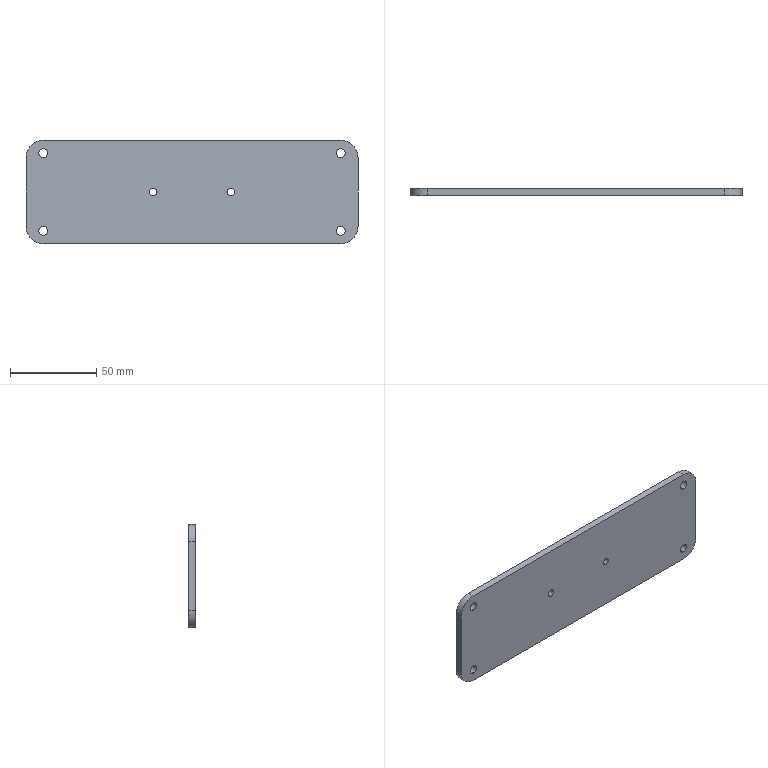Part | SolidWorks | features BaseBody 1 | 1 solid | 22 faces | box 193 x 4 x 60 mm | volume 45526 mm3 | cylinder 16 | plane 6 | commonest cylinder face diameters 5.2 x8 4.2 x4 20 x4
STEP:
#1=CARTESIAN_POINT('',(86.5,0.,-25.1));
#2=VERTEX_POINT('',#1);
#3=CARTESIAN_POINT('',(86.5,0.,-19.9));
#4=VERTEX_POINT('',#3);
#5=CARTESIAN_POINT('',(86.5,0.,-22.5));
#6=DIRECTION('',(0.,1.,0.));
#7=DIRECTION('',(0.,0.,1.));
#8=AXIS2_PLACEMENT_3D('',#5,#6,#7);
#9=CIRCLE('',#8,2.6);
#10=EDGE_CURVE('',#2,#4,#9,.T.);
#11=ORIENTED_EDGE('',*,*,#10,.F.);
#12=CARTESIAN_POINT('',(86.5,4.,-25.1));
#13=VERTEX_POINT('',#12);
#14=CARTESIAN_POINT('',(86.5,0.,-25.1));
#15=DIRECTION('',(0.,1.,0.));
#16=VECTOR('',#15,1000.);
#17=LINE('',#14,#16);
#18=EDGE_CURVE('',#2,#13,#17,.T.);
#19=ORIENTED_EDGE('',*,*,#18,.T.);
#20=CARTESIAN_POINT('',(86.5,4.,-19.9));
#21=VERTEX_POINT('',#20);
#22=CARTESIAN_POINT('',(86.5,4.,-22.5));
#23=DIRECTION('',(0.,1.,0.));
#24=DIRECTION('',(0.,0.,1.));
#25=AXIS2_PLACEMENT_3D('',#22,#23,#24);
#26=CIRCLE('',#25,2.6);
#27=EDGE_CURVE('',#13,#21,#26,.T.);
#28=ORIENTED_EDGE('',*,*,#27,.T.);
#29=CARTESIAN_POINT('',(86.5,0.,-19.9));
#30=DIRECTION('',(0.,1.,0.));
#31=VECTOR('',#30,1000.);
#32=LINE('',#29,#31);
#33=EDGE_CURVE('',#4,#21,#32,.T.);
#34=ORIENTED_EDGE('',*,*,#33,.F.);
#35=EDGE_LOOP('',(#11,#19,#28,#34));
#36=FACE_OUTER_BOUND('',#35,.T.);
#37=CARTESIAN_POINT('',(86.5,0.,-22.5));
#38=DIRECTION('',(0.,1.,0.));
#39=DIRECTION('',(0.,0.,1.));
#40=AXIS2_PLACEMENT_3D('',#37,#38,#39);
#41=CYLINDRICAL_SURFACE('',#40,2.6);
#42=ADVANCED_FACE('',(#36),#41,.F.);
#43=CARTESIAN_POINT('',(86.5,0.,19.9));
#44=VERTEX_POINT('',#43);
#45=CARTESIAN_POINT('',(86.5,0.,25.1));
#46=VERTEX_POINT('',#45);
#47=CARTESIAN_POINT('',(86.5,0.,22.5));
#48=DIRECTION('',(0.,1.,0.));
#49=DIRECTION('',(0.,0.,1.));
#50=AXIS2_PLACEMENT_3D('',#47,#48,#49);
#51=CIRCLE('',#50,2.6);
#52=EDGE_CURVE('',#44,#46,#51,.T.);
#53=ORIENTED_EDGE('',*,*,#52,.F.);
#54=CARTESIAN_POINT('',(86.5,4.,19.9));
#55=VERTEX_POINT('',#54);
#56=CARTESIAN_POINT('',(86.5,0.,19.9));
#57=DIRECTION('',(0.,1.,0.));
#58=VECTOR('',#57,1000.);
#59=LINE('',#56,#58);
#60=EDGE_CURVE('',#44,#55,#59,.T.);
#61=ORIENTED_EDGE('',*,*,#60,.T.);
#62=CARTESIAN_POINT('',(86.5,4.,25.1));
#63=VERTEX_POINT('',#62);
#64=CARTESIAN_POINT('',(86.5,4.,22.5));
#65=DIRECTION('',(0.,1.,0.));
#66=DIRECTION('',(0.,0.,1.));
#67=AXIS2_PLACEMENT_3D('',#64,#65,#66);
#68=CIRCLE('',#67,2.6);
#69=EDGE_CURVE('',#55,#63,#68,.T.);
#70=ORIENTED_EDGE('',*,*,#69,.T.);
#71=CARTESIAN_POINT('',(86.5,0.,25.1));
#72=DIRECTION('',(0.,1.,0.));
#73=VECTOR('',#72,1000.);
#74=LINE('',#71,#73);
#75=EDGE_CURVE('',#46,#63,#74,.T.);
#76=ORIENTED_EDGE('',*,*,#75,.F.);
#77=EDGE_LOOP('',(#53,#61,#70,#76));
#78=FACE_OUTER_BOUND('',#77,.T.);
#79=CARTESIAN_POINT('',(86.5,0.,22.5));
#80=DIRECTION('',(0.,1.,0.));
#81=DIRECTION('',(0.,0.,1.));
#82=AXIS2_PLACEMENT_3D('',#79,#80,#81);
#83=CYLINDRICAL_SURFACE('',#82,2.6);
#84=ADVANCED_FACE('',(#78),#83,.F.);
#85=CARTESIAN_POINT('',(-86.5,0.,19.9));
#86=VERTEX_POINT('',#85);
#87=CARTESIAN_POINT('',(-86.5,0.,25.1));
#88=VERTEX_POINT('',#87);
#89=CARTESIAN_POINT('',(-86.5,0.,22.5));
#90=DIRECTION('',(0.,1.,0.));
#91=DIRECTION('',(0.,0.,1.));
#92=AXIS2_PLACEMENT_3D('',#89,#90,#91);
#93=CIRCLE('',#92,2.6);
#94=EDGE_CURVE('',#86,#88,#93,.T.);
#95=ORIENTED_EDGE('',*,*,#94,.F.);
#96=CARTESIAN_POINT('',(-86.5,4.,19.9));
#97=VERTEX_POINT('',#96);
#98=CARTESIAN_POINT('',(-86.5,0.,19.9));
#99=DIRECTION('',(0.,1.,0.));
#100=VECTOR('',#99,1000.);
#101=LINE('',#98,#100);
#102=EDGE_CURVE('',#86,#97,#101,.T.);
#103=ORIENTED_EDGE('',*,*,#102,.T.);
#104=CARTESIAN_POINT('',(-86.5,4.,25.1));
#105=VERTEX_POINT('',#104);
#106=CARTESIAN_POINT('',(-86.5,4.,22.5));
#107=DIRECTION('',(0.,1.,0.));
#108=DIRECTION('',(0.,0.,1.));
#109=AXIS2_PLACEMENT_3D('',#106,#107,#108);
#110=CIRCLE('',#109,2.6);
#111=EDGE_CURVE('',#97,#105,#110,.T.);
#112=ORIENTED_EDGE('',*,*,#111,.T.);
#113=CARTESIAN_POINT('',(-86.5,0.,25.1));
#114=DIRECTION('',(0.,1.,0.));
#115=VECTOR('',#114,1000.);
#116=LINE('',#113,#115);
#117=EDGE_CURVE('',#88,#105,#116,.T.);
#118=ORIENTED_EDGE('',*,*,#117,.F.);
#119=EDGE_LOOP('',(#95,#103,#112,#118));
#120=FACE_OUTER_BOUND('',#119,.T.);
#121=CARTESIAN_POINT('',(-86.5,0.,22.5));
#122=DIRECTION('',(0.,1.,0.));
#123=DIRECTION('',(0.,0.,1.));
#124=AXIS2_PLACEMENT_3D('',#121,#122,#123);
#125=CYLINDRICAL_SURFACE('',#124,2.6);
#126=ADVANCED_FACE('',(#120),#125,.F.);
#127=CARTESIAN_POINT('',(-86.5,0.,-25.1));
#128=VERTEX_POINT('',#127);
#129=CARTESIAN_POINT('',(-86.5,0.,-19.9));
#130=VERTEX_POINT('',#129);
#131=CARTESIAN_POINT('',(-86.5,0.,-22.5));
#132=DIRECTION('',(0.,1.,0.));
#133=DIRECTION('',(0.,0.,1.));
#134=AXIS2_PLACEMENT_3D('',#131,#132,#133);
#135=CIRCLE('',#134,2.6);
#136=EDGE_CURVE('',#128,#130,#135,.T.);
#137=ORIENTED_EDGE('',*,*,#136,.F.);
#138=CARTESIAN_POINT('',(-86.5,4.,-25.1));
#139=VERTEX_POINT('',#138);
#140=CARTESIAN_POINT('',(-86.5,0.,-25.1));
#141=DIRECTION('',(0.,1.,0.));
#142=VECTOR('',#141,1000.);
#143=LINE('',#140,#142);
#144=EDGE_CURVE('',#128,#139,#143,.T.);
#145=ORIENTED_EDGE('',*,*,#144,.T.);
#146=CARTESIAN_POINT('',(-86.5,4.,-19.9));
#147=VERTEX_POINT('',#146);
#148=CARTESIAN_POINT('',(-86.5,4.,-22.5));
#149=DIRECTION('',(0.,1.,0.));
#150=DIRECTION('',(0.,0.,1.));
#151=AXIS2_PLACEMENT_3D('',#148,#149,#150);
#152=CIRCLE('',#151,2.6);
#153=EDGE_CURVE('',#139,#147,#152,.T.);
#154=ORIENTED_EDGE('',*,*,#153,.T.);
#155=CARTESIAN_POINT('',(-86.5,0.,-19.9));
#156=DIRECTION('',(0.,1.,0.));
#157=VECTOR('',#156,1000.);
#158=LINE('',#155,#157);
#159=EDGE_CURVE('',#130,#147,#158,.T.);
#160=ORIENTED_EDGE('',*,*,#159,.F.);
#161=EDGE_LOOP('',(#137,#145,#154,#160));
#162=FACE_OUTER_BOUND('',#161,.T.);
#163=CARTESIAN_POINT('',(-86.5,0.,-22.5));
#164=DIRECTION('',(0.,1.,0.));
#165=DIRECTION('',(0.,0.,1.));
#166=AXIS2_PLACEMENT_3D('',#163,#164,#165);
#167=CYLINDRICAL_SURFACE('',#166,2.6);
#168=ADVANCED_FACE('',(#162),#167,.F.);
#169=CARTESIAN_POINT('',(-22.5,0.,-2.1));
#170=VERTEX_POINT('',#169);
#171=CARTESIAN_POINT('',(-22.5,0.,2.1));
#172=VERTEX_POINT('',#171);
#173=CARTESIAN_POINT('',(-22.5,0.,0.));
#174=DIRECTION('',(0.,1.,0.));
#175=DIRECTION('',(0.,0.,1.));
#176=AXIS2_PLACEMENT_3D('',#173,#174,#175);
#177=CIRCLE('',#176,2.1);
#178=EDGE_CURVE('',#170,#172,#177,.T.);
#179=ORIENTED_EDGE('',*,*,#178,.F.);
#180=CARTESIAN_POINT('',(-22.5,4.,-2.1));
#181=VERTEX_POINT('',#180);
#182=CARTESIAN_POINT('',(-22.5,0.,-2.1));
#183=DIRECTION('',(0.,1.,0.));
#184=VECTOR('',#183,1000.);
#185=LINE('',#182,#184);
#186=EDGE_CURVE('',#170,#181,#185,.T.);
#187=ORIENTED_EDGE('',*,*,#186,.T.);
#188=CARTESIAN_POINT('',(-22.5,4.,2.1));
#189=VERTEX_POINT('',#188);
#190=CARTESIAN_POINT('',(-22.5,4.,0.));
#191=DIRECTION('',(0.,1.,0.));
#192=DIRECTION('',(0.,0.,1.));
#193=AXIS2_PLACEMENT_3D('',#190,#191,#192);
#194=CIRCLE('',#193,2.1);
#195=EDGE_CURVE('',#181,#189,#194,.T.);
#196=ORIENTED_EDGE('',*,*,#195,.T.);
#197=CARTESIAN_POINT('',(-22.5,0.,2.1));
#198=DIRECTION('',(0.,1.,0.));
#199=VECTOR('',#198,1000.);
#200=LINE('',#197,#199);
#201=EDGE_CURVE('',#172,#189,#200,.T.);
#202=ORIENTED_EDGE('',*,*,#201,.F.);
#203=EDGE_LOOP('',(#179,#187,#196,#202));
#204=FACE_OUTER_BOUND('',#203,.T.);
#205=CARTESIAN_POINT('',(-22.5,0.,0.));
#206=DIRECTION('',(0.,1.,0.));
#207=DIRECTION('',(0.,0.,1.));
#208=AXIS2_PLACEMENT_3D('',#205,#206,#207);
#209=CYLINDRICAL_SURFACE('',#208,2.1);
#210=ADVANCED_FACE('',(#204),#209,.F.);
#211=CARTESIAN_POINT('',(22.5,0.,-2.1));
#212=VERTEX_POINT('',#211);
#213=CARTESIAN_POINT('',(22.5,0.,2.1));
#214=VERTEX_POINT('',#213);
#215=CARTESIAN_POINT('',(22.5,0.,0.));
#216=DIRECTION('',(0.,1.,0.));
#217=DIRECTION('',(0.,0.,1.));
#218=AXIS2_PLACEMENT_3D('',#215,#216,#217);
#219=CIRCLE('',#218,2.1);
#220=EDGE_CURVE('',#212,#214,#219,.T.);
#221=ORIENTED_EDGE('',*,*,#220,.F.);
#222=CARTESIAN_POINT('',(22.5,4.,-2.1));
#223=VERTEX_POINT('',#222);
#224=CARTESIAN_POINT('',(22.5,0.,-2.1));
#225=DIRECTION('',(0.,1.,0.));
#226=VECTOR('',#225,1000.);
#227=LINE('',#224,#226);
#228=EDGE_CURVE('',#212,#223,#227,.T.);
#229=ORIENTED_EDGE('',*,*,#228,.T.);
#230=CARTESIAN_POINT('',(22.5,4.,2.1));
#231=VERTEX_POINT('',#230);
#232=CARTESIAN_POINT('',(22.5,4.,0.));
#233=DIRECTION('',(0.,1.,0.));
#234=DIRECTION('',(0.,0.,1.));
#235=AXIS2_PLACEMENT_3D('',#232,#233,#234);
#236=CIRCLE('',#235,2.1);
#237=EDGE_CURVE('',#223,#231,#236,.T.);
#238=ORIENTED_EDGE('',*,*,#237,.T.);
#239=CARTESIAN_POINT('',(22.5,0.,2.1));
#240=DIRECTION('',(0.,1.,0.));
#241=VECTOR('',#240,1000.);
#242=LINE('',#239,#241);
#243=EDGE_CURVE('',#214,#231,#242,.T.);
#244=ORIENTED_EDGE('',*,*,#243,.F.);
#245=EDGE_LOOP('',(#221,#229,#238,#244));
#246=FACE_OUTER_BOUND('',#245,.T.);
#247=CARTESIAN_POINT('',(22.5,0.,0.));
#248=DIRECTION('',(0.,1.,0.));
#249=DIRECTION('',(0.,0.,1.));
#250=AXIS2_PLACEMENT_3D('',#247,#248,#249);
#251=CYLINDRICAL_SURFACE('',#250,2.1);
#252=ADVANCED_FACE('',(#246),#251,.F.);
#253=CARTESIAN_POINT('',(96.5,4.,20.));
#254=VERTEX_POINT('',#253);
#255=CARTESIAN_POINT('',(86.5,4.,30.));
#256=VERTEX_POINT('',#255);
#257=CARTESIAN_POINT('',(86.5,4.,20.));
#258=DIRECTION('',(0.,-1.,0.));
#259=DIRECTION('',(0.,0.,-1.));
#260=AXIS2_PLACEMENT_3D('',#257,#258,#259);
#261=CIRCLE('',#260,10.);
#262=EDGE_CURVE('',#254,#256,#261,.T.);
#263=ORIENTED_EDGE('',*,*,#262,.F.);
#264=CARTESIAN_POINT('',(96.5,4.,-20.));
#265=VERTEX_POINT('',#264);
#266=CARTESIAN_POINT('',(96.5,4.,0.));
#267=DIRECTION('',(0.,0.,1.));
#268=VECTOR('',#267,1000.);
#269=LINE('',#266,#268);
#270=EDGE_CURVE('',#265,#254,#269,.T.);
#271=ORIENTED_EDGE('',*,*,#270,.F.);
#272=CARTESIAN_POINT('',(86.5,4.,-30.));
#273=VERTEX_POINT('',#272);
#274=CARTESIAN_POINT('',(86.5,4.,-20.));
#275=DIRECTION('',(0.,-1.,0.));
#276=DIRECTION('',(0.,0.,-1.));
#277=AXIS2_PLACEMENT_3D('',#274,#275,#276);
#278=CIRCLE('',#277,10.);
#279=EDGE_CURVE('',#273,#265,#278,.T.);
#280=ORIENTED_EDGE('',*,*,#279,.F.);
#281=CARTESIAN_POINT('',(-86.5,4.,-30.));
#282=VERTEX_POINT('',#281);
#283=CARTESIAN_POINT('',(0.,4.,-30.));
#284=DIRECTION('',(1.,0.,0.));
#285=VECTOR('',#284,1000.);
#286=LINE('',#283,#285);
#287=EDGE_CURVE('',#282,#273,#286,.T.);
#288=ORIENTED_EDGE('',*,*,#287,.F.);
#289=CARTESIAN_POINT('',(-96.5,4.,-20.));
#290=VERTEX_POINT('',#289);
#291=CARTESIAN_POINT('',(-86.5,4.,-20.));
#292=DIRECTION('',(0.,-1.,0.));
#293=DIRECTION('',(0.,0.,-1.));
#294=AXIS2_PLACEMENT_3D('',#291,#292,#293);
#295=CIRCLE('',#294,10.);
#296=EDGE_CURVE('',#290,#282,#295,.T.);
#297=ORIENTED_EDGE('',*,*,#296,.F.);
#298=CARTESIAN_POINT('',(-96.5,4.,20.));
#299=VERTEX_POINT('',#298);
#300=CARTESIAN_POINT('',(-96.5,4.,0.));
#301=DIRECTION('',(0.,0.,-1.));
#302=VECTOR('',#301,1000.);
#303=LINE('',#300,#302);
#304=EDGE_CURVE('',#299,#290,#303,.T.);
#305=ORIENTED_EDGE('',*,*,#304,.F.);
#306=CARTESIAN_POINT('',(-86.5,4.,30.));
#307=VERTEX_POINT('',#306);
#308=CARTESIAN_POINT('',(-86.5,4.,20.));
#309=DIRECTION('',(0.,-1.,0.));
#310=DIRECTION('',(0.,0.,-1.));
#311=AXIS2_PLACEMENT_3D('',#308,#309,#310);
#312=CIRCLE('',#311,10.);
#313=EDGE_CURVE('',#307,#299,#312,.T.);
#314=ORIENTED_EDGE('',*,*,#313,.F.);
#315=CARTESIAN_POINT('',(0.,4.,30.));
#316=DIRECTION('',(-1.,0.,0.));
#317=VECTOR('',#316,1000.);
#318=LINE('',#315,#317);
#319=EDGE_CURVE('',#256,#307,#318,.T.);
#320=ORIENTED_EDGE('',*,*,#319,.F.);
#321=EDGE_LOOP('',(#263,#271,#280,#288,#297,#305,#314,#320));
#322=FACE_OUTER_BOUND('',#321,.T.);
#323=CARTESIAN_POINT('',(86.5,4.,-22.5));
#324=DIRECTION('',(0.,1.,0.));
#325=DIRECTION('',(0.,0.,1.));
#326=AXIS2_PLACEMENT_3D('',#323,#324,#325);
#327=CIRCLE('',#326,2.6);
#328=EDGE_CURVE('',#21,#13,#327,.T.);
#329=ORIENTED_EDGE('',*,*,#328,.F.);
#330=ORIENTED_EDGE('',*,*,#27,.F.);
#331=EDGE_LOOP('',(#329,#330));
#332=FACE_BOUND('',#331,.T.);
#333=CARTESIAN_POINT('',(86.5,4.,22.5));
#334=DIRECTION('',(0.,1.,0.));
#335=DIRECTION('',(0.,0.,1.));
#336=AXIS2_PLACEMENT_3D('',#333,#334,#335);
#337=CIRCLE('',#336,2.6);
#338=EDGE_CURVE('',#63,#55,#337,.T.);
#339=ORIENTED_EDGE('',*,*,#338,.F.);
#340=ORIENTED_EDGE('',*,*,#69,.F.);
#341=EDGE_LOOP('',(#339,#340));
#342=FACE_BOUND('',#341,.T.);
#343=CARTESIAN_POINT('',(-86.5,4.,22.5));
#344=DIRECTION('',(0.,1.,0.));
#345=DIRECTION('',(0.,0.,1.));
#346=AXIS2_PLACEMENT_3D('',#343,#344,#345);
#347=CIRCLE('',#346,2.6);
#348=EDGE_CURVE('',#105,#97,#347,.T.);
#349=ORIENTED_EDGE('',*,*,#348,.F.);
#350=ORIENTED_EDGE('',*,*,#111,.F.);
#351=EDGE_LOOP('',(#349,#350));
#352=FACE_BOUND('',#351,.T.);
#353=CARTESIAN_POINT('',(-86.5,4.,-22.5));
#354=DIRECTION('',(0.,1.,0.));
#355=DIRECTION('',(0.,0.,1.));
#356=AXIS2_PLACEMENT_3D('',#353,#354,#355);
#357=CIRCLE('',#356,2.6);
#358=EDGE_CURVE('',#147,#139,#357,.T.);
#359=ORIENTED_EDGE('',*,*,#358,.F.);
#360=ORIENTED_EDGE('',*,*,#153,.F.);
#361=EDGE_LOOP('',(#359,#360));
#362=FACE_BOUND('',#361,.T.);
#363=CARTESIAN_POINT('',(-22.5,4.,0.));
#364=DIRECTION('',(0.,1.,0.));
#365=DIRECTION('',(0.,0.,1.));
#366=AXIS2_PLACEMENT_3D('',#363,#364,#365);
#367=CIRCLE('',#366,2.1);
#368=EDGE_CURVE('',#189,#181,#367,.T.);
#369=ORIENTED_EDGE('',*,*,#368,.F.);
#370=ORIENTED_EDGE('',*,*,#195,.F.);
#371=EDGE_LOOP('',(#369,#370));
#372=FACE_BOUND('',#371,.T.);
#373=CARTESIAN_POINT('',(22.5,4.,0.));
#374=DIRECTION('',(0.,1.,0.));
#375=DIRECTION('',(0.,0.,1.));
#376=AXIS2_PLACEMENT_3D('',#373,#374,#375);
#377=CIRCLE('',#376,2.1);
#378=EDGE_CURVE('',#231,#223,#377,.T.);
#379=ORIENTED_EDGE('',*,*,#378,.F.);
#380=ORIENTED_EDGE('',*,*,#237,.F.);
#381=EDGE_LOOP('',(#379,#380));
#382=FACE_BOUND('',#381,.T.);
#383=CARTESIAN_POINT('',(0.,4.,0.));
#384=DIRECTION('',(0.,-1.,0.));
#385=DIRECTION('',(0.,0.,-1.));
#386=AXIS2_PLACEMENT_3D('',#383,#384,#385);
#387=PLANE('',#386);
#388=ADVANCED_FACE('',(#322,#332,#342,#352,#362,#372,#382),#387,.F.);
#389=CARTESIAN_POINT('',(86.5,0.,30.));
#390=VERTEX_POINT('',#389);
#391=CARTESIAN_POINT('',(86.5,4.,30.));
#392=DIRECTION('',(0.,-1.,0.));
#393=VECTOR('',#392,1000.);
#394=LINE('',#391,#393);
#395=EDGE_CURVE('',#256,#390,#394,.T.);
#396=ORIENTED_EDGE('',*,*,#395,.F.);
#397=ORIENTED_EDGE('',*,*,#319,.T.);
#398=CARTESIAN_POINT('',(-86.5,0.,30.));
#399=VERTEX_POINT('',#398);
#400=CARTESIAN_POINT('',(-86.5,4.,30.));
#401=DIRECTION('',(0.,1.,0.));
#402=VECTOR('',#401,1000.);
#403=LINE('',#400,#402);
#404=EDGE_CURVE('',#399,#307,#403,.T.);
#405=ORIENTED_EDGE('',*,*,#404,.F.);
#406=CARTESIAN_POINT('',(-96.5,0.,30.));
#407=DIRECTION('',(-1.,0.,0.));
#408=VECTOR('',#407,1000.);
#409=LINE('',#406,#408);
#410=EDGE_CURVE('',#390,#399,#409,.T.);
#411=ORIENTED_EDGE('',*,*,#410,.F.);
#412=EDGE_LOOP('',(#396,#397,#405,#411));
#413=FACE_OUTER_BOUND('',#412,.T.);
#414=CARTESIAN_POINT('',(-96.5,4.,30.));
#415=DIRECTION('',(0.,0.,-1.));
#416=DIRECTION('',(-1.,0.,0.));
#417=AXIS2_PLACEMENT_3D('',#414,#415,#416);
#418=PLANE('',#417);
#419=ADVANCED_FACE('',(#413),#418,.F.);
#420=CARTESIAN_POINT('',(96.5,0.,20.));
#421=VERTEX_POINT('',#420);
#422=CARTESIAN_POINT('',(86.5,0.,20.));
#423=DIRECTION('',(0.,1.,0.));
#424=DIRECTION('',(0.,0.,-1.));
#425=AXIS2_PLACEMENT_3D('',#422,#423,#424);
#426=CIRCLE('',#425,10.);
#427=EDGE_CURVE('',#390,#421,#426,.T.);
#428=ORIENTED_EDGE('',*,*,#427,.T.);
#429=CARTESIAN_POINT('',(96.5,4.,20.));
#430=DIRECTION('',(0.,1.,0.));
#431=VECTOR('',#430,1000.);
#432=LINE('',#429,#431);
#433=EDGE_CURVE('',#421,#254,#432,.T.);
#434=ORIENTED_EDGE('',*,*,#433,.T.);
#435=ORIENTED_EDGE('',*,*,#262,.T.);
#436=ORIENTED_EDGE('',*,*,#395,.T.);
#437=EDGE_LOOP('',(#428,#434,#435,#436));
#438=FACE_OUTER_BOUND('',#437,.T.);
#439=CARTESIAN_POINT('',(86.5,4.,20.));
#440=DIRECTION('',(0.,-1.,0.));
#441=DIRECTION('',(0.,0.,-1.));
#442=AXIS2_PLACEMENT_3D('',#439,#440,#441);
#443=CYLINDRICAL_SURFACE('',#442,10.);
#444=ADVANCED_FACE('',(#438),#443,.T.);
#445=ORIENTED_EDGE('',*,*,#433,.F.);
#446=CARTESIAN_POINT('',(96.5,0.,-20.));
#447=VERTEX_POINT('',#446);
#448=CARTESIAN_POINT('',(96.5,0.,30.));
#449=DIRECTION('',(0.,0.,1.));
#450=VECTOR('',#449,1000.);
#451=LINE('',#448,#450);
#452=EDGE_CURVE('',#447,#421,#451,.T.);
#453=ORIENTED_EDGE('',*,*,#452,.F.);
#454=CARTESIAN_POINT('',(96.5,4.,-20.));
#455=DIRECTION('',(0.,-1.,0.));
#456=VECTOR('',#455,1000.);
#457=LINE('',#454,#456);
#458=EDGE_CURVE('',#265,#447,#457,.T.);
#459=ORIENTED_EDGE('',*,*,#458,.F.);
#460=ORIENTED_EDGE('',*,*,#270,.T.);
#461=EDGE_LOOP('',(#445,#453,#459,#460));
#462=FACE_OUTER_BOUND('',#461,.T.);
#463=CARTESIAN_POINT('',(96.5,4.,30.));
#464=DIRECTION('',(-1.,0.,0.));
#465=DIRECTION('',(0.,0.,1.));
#466=AXIS2_PLACEMENT_3D('',#463,#464,#465);
#467=PLANE('',#466);
#468=ADVANCED_FACE('',(#462),#467,.F.);
#469=CARTESIAN_POINT('',(86.5,0.,-30.));
#470=VERTEX_POINT('',#469);
#471=CARTESIAN_POINT('',(86.5,0.,-20.));
#472=DIRECTION('',(0.,1.,0.));
#473=DIRECTION('',(0.,0.,-1.));
#474=AXIS2_PLACEMENT_3D('',#471,#472,#473);
#475=CIRCLE('',#474,10.);
#476=EDGE_CURVE('',#447,#470,#475,.T.);
#477=ORIENTED_EDGE('',*,*,#476,.T.);
#478=CARTESIAN_POINT('',(86.5,4.,-30.));
#479=DIRECTION('',(0.,1.,0.));
#480=VECTOR('',#479,1000.);
#481=LINE('',#478,#480);
#482=EDGE_CURVE('',#470,#273,#481,.T.);
#483=ORIENTED_EDGE('',*,*,#482,.T.);
#484=ORIENTED_EDGE('',*,*,#279,.T.);
#485=ORIENTED_EDGE('',*,*,#458,.T.);
#486=EDGE_LOOP('',(#477,#483,#484,#485));
#487=FACE_OUTER_BOUND('',#486,.T.);
#488=CARTESIAN_POINT('',(86.5,4.,-20.));
#489=DIRECTION('',(0.,-1.,0.));
#490=DIRECTION('',(0.,0.,-1.));
#491=AXIS2_PLACEMENT_3D('',#488,#489,#490);
#492=CYLINDRICAL_SURFACE('',#491,10.);
#493=ADVANCED_FACE('',(#487),#492,.T.);
#494=ORIENTED_EDGE('',*,*,#482,.F.);
#495=CARTESIAN_POINT('',(-86.5,0.,-30.));
#496=VERTEX_POINT('',#495);
#497=CARTESIAN_POINT('',(-96.5,0.,-30.));
#498=DIRECTION('',(1.,0.,0.));
#499=VECTOR('',#498,1000.);
#500=LINE('',#497,#499);
#501=EDGE_CURVE('',#496,#470,#500,.T.);
#502=ORIENTED_EDGE('',*,*,#501,.F.);
#503=CARTESIAN_POINT('',(-86.5,4.,-30.));
#504=DIRECTION('',(0.,-1.,0.));
#505=VECTOR('',#504,1000.);
#506=LINE('',#503,#505);
#507=EDGE_CURVE('',#282,#496,#506,.T.);
#508=ORIENTED_EDGE('',*,*,#507,.F.);
#509=ORIENTED_EDGE('',*,*,#287,.T.);
#510=EDGE_LOOP('',(#494,#502,#508,#509));
#511=FACE_OUTER_BOUND('',#510,.T.);
#512=CARTESIAN_POINT('',(-96.5,4.,-30.));
#513=DIRECTION('',(0.,0.,1.));
#514=DIRECTION('',(1.,0.,0.));
#515=AXIS2_PLACEMENT_3D('',#512,#513,#514);
#516=PLANE('',#515);
#517=ADVANCED_FACE('',(#511),#516,.F.);
#518=CARTESIAN_POINT('',(-96.5,0.,-20.));
#519=VERTEX_POINT('',#518);
#520=CARTESIAN_POINT('',(-86.5,0.,-20.));
#521=DIRECTION('',(0.,1.,0.));
#522=DIRECTION('',(0.,0.,-1.));
#523=AXIS2_PLACEMENT_3D('',#520,#521,#522);
#524=CIRCLE('',#523,10.);
#525=EDGE_CURVE('',#496,#519,#524,.T.);
#526=ORIENTED_EDGE('',*,*,#525,.T.);
#527=CARTESIAN_POINT('',(-96.5,4.,-20.));
#528=DIRECTION('',(0.,1.,0.));
#529=VECTOR('',#528,1000.);
#530=LINE('',#527,#529);
#531=EDGE_CURVE('',#519,#290,#530,.T.);
#532=ORIENTED_EDGE('',*,*,#531,.T.);
#533=ORIENTED_EDGE('',*,*,#296,.T.);
#534=ORIENTED_EDGE('',*,*,#507,.T.);
#535=EDGE_LOOP('',(#526,#532,#533,#534));
#536=FACE_OUTER_BOUND('',#535,.T.);
#537=CARTESIAN_POINT('',(-86.5,4.,-20.));
#538=DIRECTION('',(0.,-1.,0.));
#539=DIRECTION('',(0.,0.,-1.));
#540=AXIS2_PLACEMENT_3D('',#537,#538,#539);
#541=CYLINDRICAL_SURFACE('',#540,10.);
#542=ADVANCED_FACE('',(#536),#541,.T.);
#543=CARTESIAN_POINT('',(-96.5,0.,20.));
#544=VERTEX_POINT('',#543);
#545=CARTESIAN_POINT('',(-96.5,4.,20.));
#546=DIRECTION('',(0.,-1.,0.));
#547=VECTOR('',#546,1000.);
#548=LINE('',#545,#547);
#549=EDGE_CURVE('',#299,#544,#548,.T.);
#550=ORIENTED_EDGE('',*,*,#549,.F.);
#551=ORIENTED_EDGE('',*,*,#304,.T.);
#552=ORIENTED_EDGE('',*,*,#531,.F.);
#553=CARTESIAN_POINT('',(-96.5,0.,30.));
#554=DIRECTION('',(0.,0.,-1.));
#555=VECTOR('',#554,1000.);
#556=LINE('',#553,#555);
#557=EDGE_CURVE('',#544,#519,#556,.T.);
#558=ORIENTED_EDGE('',*,*,#557,.F.);
#559=EDGE_LOOP('',(#550,#551,#552,#558));
#560=FACE_OUTER_BOUND('',#559,.T.);
#561=CARTESIAN_POINT('',(-96.5,4.,30.));
#562=DIRECTION('',(1.,0.,0.));
#563=DIRECTION('',(0.,0.,-1.));
#564=AXIS2_PLACEMENT_3D('',#561,#562,#563);
#565=PLANE('',#564);
#566=ADVANCED_FACE('',(#560),#565,.F.);
#567=CARTESIAN_POINT('',(-86.5,0.,20.));
#568=DIRECTION('',(0.,1.,0.));
#569=DIRECTION('',(0.,0.,-1.));
#570=AXIS2_PLACEMENT_3D('',#567,#568,#569);
#571=CIRCLE('',#570,10.);
#572=EDGE_CURVE('',#544,#399,#571,.T.);
#573=ORIENTED_EDGE('',*,*,#572,.T.);
#574=ORIENTED_EDGE('',*,*,#404,.T.);
#575=ORIENTED_EDGE('',*,*,#313,.T.);
#576=ORIENTED_EDGE('',*,*,#549,.T.);
#577=EDGE_LOOP('',(#573,#574,#575,#576));
#578=FACE_OUTER_BOUND('',#577,.T.);
#579=CARTESIAN_POINT('',(-86.5,4.,20.));
#580=DIRECTION('',(0.,-1.,0.));
#581=DIRECTION('',(0.,0.,-1.));
#582=AXIS2_PLACEMENT_3D('',#579,#580,#581);
#583=CYLINDRICAL_SURFACE('',#582,10.);
#584=ADVANCED_FACE('',(#578),#583,.T.);
#585=ORIENTED_EDGE('',*,*,#18,.F.);
#586=CARTESIAN_POINT('',(86.5,0.,-22.5));
#587=DIRECTION('',(0.,1.,0.));
#588=DIRECTION('',(0.,0.,1.));
#589=AXIS2_PLACEMENT_3D('',#586,#587,#588);
#590=CIRCLE('',#589,2.6);
#591=EDGE_CURVE('',#4,#2,#590,.T.);
#592=ORIENTED_EDGE('',*,*,#591,.F.);
#593=ORIENTED_EDGE('',*,*,#33,.T.);
#594=ORIENTED_EDGE('',*,*,#328,.T.);
#595=EDGE_LOOP('',(#585,#592,#593,#594));
#596=FACE_OUTER_BOUND('',#595,.T.);
#597=CARTESIAN_POINT('',(86.5,0.,-22.5));
#598=DIRECTION('',(0.,1.,0.));
#599=DIRECTION('',(0.,0.,1.));
#600=AXIS2_PLACEMENT_3D('',#597,#598,#599);
#601=CYLINDRICAL_SURFACE('',#600,2.6);
#602=ADVANCED_FACE('',(#596),#601,.F.);
#603=ORIENTED_EDGE('',*,*,#60,.F.);
#604=CARTESIAN_POINT('',(86.5,0.,22.5));
#605=DIRECTION('',(0.,1.,0.));
#606=DIRECTION('',(0.,0.,1.));
#607=AXIS2_PLACEMENT_3D('',#604,#605,#606);
#608=CIRCLE('',#607,2.6);
#609=EDGE_CURVE('',#46,#44,#608,.T.);
#610=ORIENTED_EDGE('',*,*,#609,.F.);
#611=ORIENTED_EDGE('',*,*,#75,.T.);
#612=ORIENTED_EDGE('',*,*,#338,.T.);
#613=EDGE_LOOP('',(#603,#610,#611,#612));
#614=FACE_OUTER_BOUND('',#613,.T.);
#615=CARTESIAN_POINT('',(86.5,0.,22.5));
#616=DIRECTION('',(0.,1.,0.));
#617=DIRECTION('',(0.,0.,1.));
#618=AXIS2_PLACEMENT_3D('',#615,#616,#617);
#619=CYLINDRICAL_SURFACE('',#618,2.6);
#620=ADVANCED_FACE('',(#614),#619,.F.);
#621=ORIENTED_EDGE('',*,*,#102,.F.);
#622=CARTESIAN_POINT('',(-86.5,0.,22.5));
#623=DIRECTION('',(0.,1.,0.));
#624=DIRECTION('',(0.,0.,1.));
#625=AXIS2_PLACEMENT_3D('',#622,#623,#624);
#626=CIRCLE('',#625,2.6);
#627=EDGE_CURVE('',#88,#86,#626,.T.);
#628=ORIENTED_EDGE('',*,*,#627,.F.);
#629=ORIENTED_EDGE('',*,*,#117,.T.);
#630=ORIENTED_EDGE('',*,*,#348,.T.);
#631=EDGE_LOOP('',(#621,#628,#629,#630));
#632=FACE_OUTER_BOUND('',#631,.T.);
#633=CARTESIAN_POINT('',(-86.5,0.,22.5));
#634=DIRECTION('',(0.,1.,0.));
#635=DIRECTION('',(0.,0.,1.));
#636=AXIS2_PLACEMENT_3D('',#633,#634,#635);
#637=CYLINDRICAL_SURFACE('',#636,2.6);
#638=ADVANCED_FACE('',(#632),#637,.F.);
#639=ORIENTED_EDGE('',*,*,#144,.F.);
#640=CARTESIAN_POINT('',(-86.5,0.,-22.5));
#641=DIRECTION('',(0.,1.,0.));
#642=DIRECTION('',(0.,0.,1.));
#643=AXIS2_PLACEMENT_3D('',#640,#641,#642);
#644=CIRCLE('',#643,2.6);
#645=EDGE_CURVE('',#130,#128,#644,.T.);
#646=ORIENTED_EDGE('',*,*,#645,.F.);
#647=ORIENTED_EDGE('',*,*,#159,.T.);
#648=ORIENTED_EDGE('',*,*,#358,.T.);
#649=EDGE_LOOP('',(#639,#646,#647,#648));
#650=FACE_OUTER_BOUND('',#649,.T.);
#651=CARTESIAN_POINT('',(-86.5,0.,-22.5));
#652=DIRECTION('',(0.,1.,0.));
#653=DIRECTION('',(0.,0.,1.));
#654=AXIS2_PLACEMENT_3D('',#651,#652,#653);
#655=CYLINDRICAL_SURFACE('',#654,2.6);
#656=ADVANCED_FACE('',(#650),#655,.F.);
#657=ORIENTED_EDGE('',*,*,#186,.F.);
#658=CARTESIAN_POINT('',(-22.5,0.,0.));
#659=DIRECTION('',(0.,1.,0.));
#660=DIRECTION('',(0.,0.,1.));
#661=AXIS2_PLACEMENT_3D('',#658,#659,#660);
#662=CIRCLE('',#661,2.1);
#663=EDGE_CURVE('',#172,#170,#662,.T.);
#664=ORIENTED_EDGE('',*,*,#663,.F.);
#665=ORIENTED_EDGE('',*,*,#201,.T.);
#666=ORIENTED_EDGE('',*,*,#368,.T.);
#667=EDGE_LOOP('',(#657,#664,#665,#666));
#668=FACE_OUTER_BOUND('',#667,.T.);
#669=CARTESIAN_POINT('',(-22.5,0.,0.));
#670=DIRECTION('',(0.,1.,0.));
#671=DIRECTION('',(0.,0.,1.));
#672=AXIS2_PLACEMENT_3D('',#669,#670,#671);
#673=CYLINDRICAL_SURFACE('',#672,2.1);
#674=ADVANCED_FACE('',(#668),#673,.F.);
#675=ORIENTED_EDGE('',*,*,#228,.F.);
#676=CARTESIAN_POINT('',(22.5,0.,0.));
#677=DIRECTION('',(0.,1.,0.));
#678=DIRECTION('',(0.,0.,1.));
#679=AXIS2_PLACEMENT_3D('',#676,#677,#678);
#680=CIRCLE('',#679,2.1);
#681=EDGE_CURVE('',#214,#212,#680,.T.);
#682=ORIENTED_EDGE('',*,*,#681,.F.);
#683=ORIENTED_EDGE('',*,*,#243,.T.);
#684=ORIENTED_EDGE('',*,*,#378,.T.);
#685=EDGE_LOOP('',(#675,#682,#683,#684));
#686=FACE_OUTER_BOUND('',#685,.T.);
#687=CARTESIAN_POINT('',(22.5,0.,0.));
#688=DIRECTION('',(0.,1.,0.));
#689=DIRECTION('',(0.,0.,1.));
#690=AXIS2_PLACEMENT_3D('',#687,#688,#689);
#691=CYLINDRICAL_SURFACE('',#690,2.1);
#692=ADVANCED_FACE('',(#686),#691,.F.);
#693=ORIENTED_EDGE('',*,*,#501,.T.);
#694=ORIENTED_EDGE('',*,*,#476,.F.);
#695=ORIENTED_EDGE('',*,*,#452,.T.);
#696=ORIENTED_EDGE('',*,*,#427,.F.);
#697=ORIENTED_EDGE('',*,*,#410,.T.);
#698=ORIENTED_EDGE('',*,*,#572,.F.);
#699=ORIENTED_EDGE('',*,*,#557,.T.);
#700=ORIENTED_EDGE('',*,*,#525,.F.);
#701=EDGE_LOOP('',(#693,#694,#695,#696,#697,#698,#699,#700));
#702=FACE_OUTER_BOUND('',#701,.T.);
#703=ORIENTED_EDGE('',*,*,#591,.T.);
#704=ORIENTED_EDGE('',*,*,#10,.T.);
#705=EDGE_LOOP('',(#703,#704));
#706=FACE_BOUND('',#705,.T.);
#707=ORIENTED_EDGE('',*,*,#609,.T.);
#708=ORIENTED_EDGE('',*,*,#52,.T.);
#709=EDGE_LOOP('',(#707,#708));
#710=FACE_BOUND('',#709,.T.);
#711=ORIENTED_EDGE('',*,*,#627,.T.);
#712=ORIENTED_EDGE('',*,*,#94,.T.);
#713=EDGE_LOOP('',(#711,#712));
#714=FACE_BOUND('',#713,.T.);
#715=ORIENTED_EDGE('',*,*,#645,.T.);
#716=ORIENTED_EDGE('',*,*,#136,.T.);
#717=EDGE_LOOP('',(#715,#716));
#718=FACE_BOUND('',#717,.T.);
#719=ORIENTED_EDGE('',*,*,#663,.T.);
#720=ORIENTED_EDGE('',*,*,#178,.T.);
#721=EDGE_LOOP('',(#719,#720));
#722=FACE_BOUND('',#721,.T.);
#723=ORIENTED_EDGE('',*,*,#681,.T.);
#724=ORIENTED_EDGE('',*,*,#220,.T.);
#725=EDGE_LOOP('',(#723,#724));
#726=FACE_BOUND('',#725,.T.);
#727=CARTESIAN_POINT('',(0.,0.,0.));
#728=DIRECTION('',(0.,-1.,0.));
#729=DIRECTION('',(0.,0.,-1.));
#730=AXIS2_PLACEMENT_3D('',#727,#728,#729);
#731=PLANE('',#730);
#732=ADVANCED_FACE('',(#702,#706,#710,#714,#718,#722,#726),#731,.T.);
#733=CLOSED_SHELL('',(#42,#84,#126,#168,#210,#252,#388,#419,#444,#468,#493,#517,#542,#566,#584,#602,#620,#638,#656,#674,#692,#732));
#734=MANIFOLD_SOLID_BREP('',#733);
#735=CARTESIAN_POINT('',(0.,0.,0.));
#736=DIRECTION('',(0.,0.,1.));
#737=DIRECTION('',(1.,0.,0.));
#738=AXIS2_PLACEMENT_3D('',#735,#736,#737);
#739=(LENGTH_UNIT()NAMED_UNIT(*)SI_UNIT(.MILLI.,.METRE.));
#740=UNCERTAINTY_MEASURE_WITH_UNIT(LENGTH_MEASURE(0.00001),#739,'','');
#741=(NAMED_UNIT(*)PLANE_ANGLE_UNIT()SI_UNIT($,.RADIAN.));
#742=(NAMED_UNIT(*)SI_UNIT($,.STERADIAN.)SOLID_ANGLE_UNIT());
#743=(GEOMETRIC_REPRESENTATION_CONTEXT(3)GLOBAL_UNCERTAINTY_ASSIGNED_CONTEXT((#740))GLOBAL_UNIT_ASSIGNED_CONTEXT((#739,#741,#742))REPRESENTATION_CONTEXT('',''));
#744=ADVANCED_BREP_SHAPE_REPRESENTATION('',(#734,#738),#743);